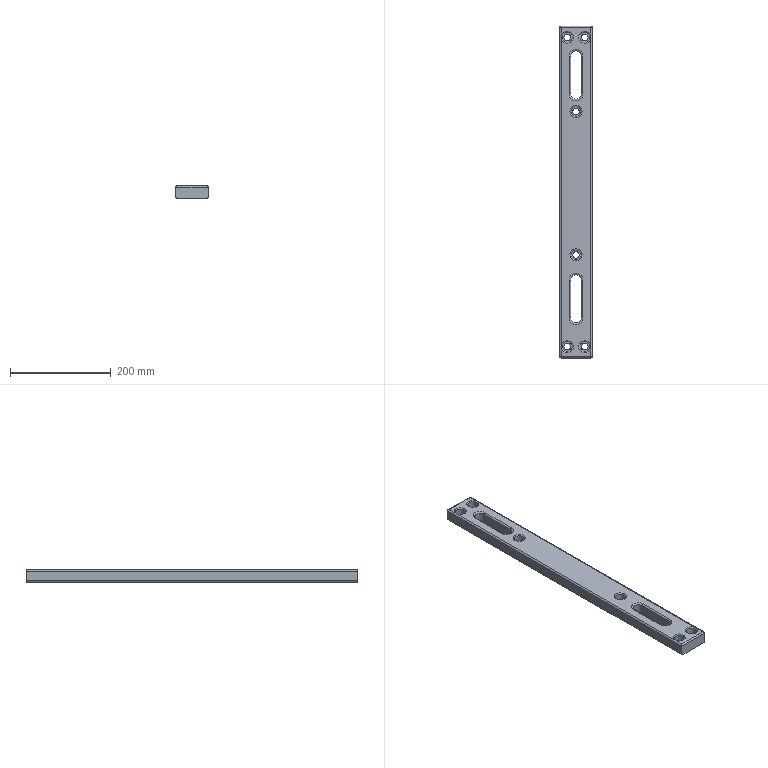Part | NX | features solid 2 | 1 solid | 53 faces | box 65 x 660 x 25 mm | volume 933665 mm3 | cylinder 26 | plane 17 | torus 10 | commonest cylinder face diameters 6 x10 13 x6 20 x6 21 x4
STEP:
#1=CARTESIAN_POINT('',(-465.,-309.,403.));
#2=VERTEX_POINT('',#1);
#3=CARTESIAN_POINT('',(-455.,-309.,403.));
#4=DIRECTION('',(0.,0.,-1.));
#5=DIRECTION('',(-1.,0.,0.));
#6=AXIS2_PLACEMENT_3D('',#3,#4,#5);
#7=CIRCLE('',#6,10.);
#8=EDGE_CURVE('',#2,#2,#7,.T.);
#9=ORIENTED_EDGE('',*,*,#8,.F.);
#10=EDGE_LOOP('',(#9));
#11=FACE_BOUND('',#10,.T.);
#12=CARTESIAN_POINT('',(-445.,-309.,390.));
#13=VERTEX_POINT('',#12);
#14=CARTESIAN_POINT('',(-455.,-309.,390.));
#15=DIRECTION('',(0.,0.,-1.));
#16=DIRECTION('',(1.,0.,0.));
#17=AXIS2_PLACEMENT_3D('',#14,#15,#16);
#18=CIRCLE('',#17,10.);
#19=EDGE_CURVE('',#13,#13,#18,.T.);
#20=ORIENTED_EDGE('',*,*,#19,.T.);
#21=EDGE_LOOP('',(#20));
#22=FACE_BOUND('',#21,.T.);
#23=CARTESIAN_POINT('',(-455.,-309.,390.));
#24=DIRECTION('',(0.,0.,1.));
#25=DIRECTION('',(1.,0.,0.));
#26=AXIS2_PLACEMENT_3D('',#23,#24,#25);
#27=CYLINDRICAL_SURFACE('',#26,10.);
#28=ADVANCED_FACE('',(#11,#22),#27,.F.);
#29=CARTESIAN_POINT('',(-500.,-309.,403.));
#30=VERTEX_POINT('',#29);
#31=CARTESIAN_POINT('',(-490.,-309.,403.));
#32=DIRECTION('',(0.,0.,-1.));
#33=DIRECTION('',(-1.,0.,0.));
#34=AXIS2_PLACEMENT_3D('',#31,#32,#33);
#35=CIRCLE('',#34,10.);
#36=EDGE_CURVE('',#30,#30,#35,.T.);
#37=ORIENTED_EDGE('',*,*,#36,.F.);
#38=EDGE_LOOP('',(#37));
#39=FACE_BOUND('',#38,.T.);
#40=CARTESIAN_POINT('',(-480.,-309.,390.));
#41=VERTEX_POINT('',#40);
#42=CARTESIAN_POINT('',(-490.,-309.,390.));
#43=DIRECTION('',(0.,0.,-1.));
#44=DIRECTION('',(1.,0.,0.));
#45=AXIS2_PLACEMENT_3D('',#42,#43,#44);
#46=CIRCLE('',#45,10.);
#47=EDGE_CURVE('',#41,#41,#46,.T.);
#48=ORIENTED_EDGE('',*,*,#47,.T.);
#49=EDGE_LOOP('',(#48));
#50=FACE_BOUND('',#49,.T.);
#51=CARTESIAN_POINT('',(-490.,-309.,390.));
#52=DIRECTION('',(0.,0.,1.));
#53=DIRECTION('',(1.,0.,0.));
#54=AXIS2_PLACEMENT_3D('',#51,#52,#53);
#55=CYLINDRICAL_SURFACE('',#54,10.);
#56=ADVANCED_FACE('',(#39,#50),#55,.F.);
#57=CARTESIAN_POINT('',(-482.5,-126.5,403.));
#58=VERTEX_POINT('',#57);
#59=CARTESIAN_POINT('',(-472.5,-126.5,403.));
#60=DIRECTION('',(0.,0.,-1.));
#61=DIRECTION('',(-1.,0.,0.));
#62=AXIS2_PLACEMENT_3D('',#59,#60,#61);
#63=CIRCLE('',#62,10.);
#64=EDGE_CURVE('',#58,#58,#63,.T.);
#65=ORIENTED_EDGE('',*,*,#64,.F.);
#66=EDGE_LOOP('',(#65));
#67=FACE_BOUND('',#66,.T.);
#68=CARTESIAN_POINT('',(-462.5,-126.5,390.));
#69=VERTEX_POINT('',#68);
#70=CARTESIAN_POINT('',(-472.5,-126.5,390.));
#71=DIRECTION('',(0.,0.,-1.));
#72=DIRECTION('',(1.,0.,0.));
#73=AXIS2_PLACEMENT_3D('',#70,#71,#72);
#74=CIRCLE('',#73,10.);
#75=EDGE_CURVE('',#69,#69,#74,.T.);
#76=ORIENTED_EDGE('',*,*,#75,.T.);
#77=EDGE_LOOP('',(#76));
#78=FACE_BOUND('',#77,.T.);
#79=CARTESIAN_POINT('',(-472.5,-126.5,390.));
#80=DIRECTION('',(0.,0.,1.));
#81=DIRECTION('',(1.,0.,0.));
#82=AXIS2_PLACEMENT_3D('',#79,#80,#81);
#83=CYLINDRICAL_SURFACE('',#82,10.);
#84=ADVANCED_FACE('',(#67,#78),#83,.F.);
#85=ORIENTED_EDGE('',*,*,#47,.F.);
#86=EDGE_LOOP('',(#85));
#87=FACE_BOUND('',#86,.T.);
#88=CARTESIAN_POINT('',(-483.5,-309.,390.));
#89=VERTEX_POINT('',#88);
#90=CARTESIAN_POINT('',(-490.,-309.,390.));
#91=DIRECTION('',(0.,0.,-1.));
#92=DIRECTION('',(1.,0.,0.));
#93=AXIS2_PLACEMENT_3D('',#90,#91,#92);
#94=CIRCLE('',#93,6.5);
#95=EDGE_CURVE('',#89,#89,#94,.F.);
#96=ORIENTED_EDGE('',*,*,#95,.F.);
#97=EDGE_LOOP('',(#96));
#98=FACE_BOUND('',#97,.T.);
#99=CARTESIAN_POINT('',(-490.,-331.5,390.));
#100=DIRECTION('',(0.,0.,1.));
#101=DIRECTION('',(1.,0.,0.));
#102=AXIS2_PLACEMENT_3D('',#99,#100,#101);
#103=PLANE('',#102);
#104=ADVANCED_FACE('',(#87,#98),#103,.T.);
#105=ORIENTED_EDGE('',*,*,#19,.F.);
#106=EDGE_LOOP('',(#105));
#107=FACE_BOUND('',#106,.T.);
#108=CARTESIAN_POINT('',(-448.5,-309.,390.));
#109=VERTEX_POINT('',#108);
#110=CARTESIAN_POINT('',(-455.,-309.,390.));
#111=DIRECTION('',(0.,0.,-1.));
#112=DIRECTION('',(1.,0.,0.));
#113=AXIS2_PLACEMENT_3D('',#110,#111,#112);
#114=CIRCLE('',#113,6.5);
#115=EDGE_CURVE('',#109,#109,#114,.F.);
#116=ORIENTED_EDGE('',*,*,#115,.F.);
#117=EDGE_LOOP('',(#116));
#118=FACE_BOUND('',#117,.T.);
#119=CARTESIAN_POINT('',(-455.,-331.5,390.));
#120=DIRECTION('',(0.,0.,1.));
#121=DIRECTION('',(1.,0.,0.));
#122=AXIS2_PLACEMENT_3D('',#119,#120,#121);
#123=PLANE('',#122);
#124=ADVANCED_FACE('',(#107,#118),#123,.T.);
#125=ORIENTED_EDGE('',*,*,#75,.F.);
#126=EDGE_LOOP('',(#125));
#127=FACE_BOUND('',#126,.T.);
#128=CARTESIAN_POINT('',(-466.,-126.5,390.));
#129=VERTEX_POINT('',#128);
#130=CARTESIAN_POINT('',(-472.5,-126.5,390.));
#131=DIRECTION('',(0.,0.,-1.));
#132=DIRECTION('',(1.,0.,0.));
#133=AXIS2_PLACEMENT_3D('',#130,#131,#132);
#134=CIRCLE('',#133,6.5);
#135=EDGE_CURVE('',#129,#129,#134,.F.);
#136=ORIENTED_EDGE('',*,*,#135,.F.);
#137=EDGE_LOOP('',(#136));
#138=FACE_BOUND('',#137,.T.);
#139=CARTESIAN_POINT('',(-472.5,-128.,390.));
#140=DIRECTION('',(0.,0.,1.));
#141=DIRECTION('',(1.,0.,0.));
#142=AXIS2_PLACEMENT_3D('',#139,#140,#141);
#143=PLANE('',#142);
#144=ADVANCED_FACE('',(#127,#138),#143,.T.);
#145=CARTESIAN_POINT('',(-443.,-309.007,405.));
#146=VERTEX_POINT('',#145);
#147=CARTESIAN_POINT('',(-455.,-309.,405.));
#148=DIRECTION('',(0.,0.,-1.));
#149=DIRECTION('',(-1.,0.,0.));
#150=AXIS2_PLACEMENT_3D('',#147,#148,#149);
#151=CIRCLE('',#150,12.);
#152=EDGE_CURVE('',#146,#146,#151,.F.);
#153=ORIENTED_EDGE('',*,*,#152,.T.);
#154=EDGE_LOOP('',(#153));
#155=FACE_BOUND('',#154,.T.);
#156=ORIENTED_EDGE('',*,*,#8,.T.);
#157=EDGE_LOOP('',(#156));
#158=FACE_BOUND('',#157,.T.);
#159=CARTESIAN_POINT('',(-455.,-309.,403.));
#160=DIRECTION('',(0.,0.,1.));
#161=DIRECTION('',(-1.,0.,0.));
#162=AXIS2_PLACEMENT_3D('',#159,#160,#161);
#163=TOROIDAL_SURFACE('',#162,12.,2.);
#164=ADVANCED_FACE('',(#155,#158),#163,.T.);
#165=CARTESIAN_POINT('',(-502.,-309.007,405.));
#166=VERTEX_POINT('',#165);
#167=CARTESIAN_POINT('',(-490.,-309.,405.));
#168=DIRECTION('',(0.,0.,-1.));
#169=DIRECTION('',(-1.,0.,0.));
#170=AXIS2_PLACEMENT_3D('',#167,#168,#169);
#171=CIRCLE('',#170,12.);
#172=EDGE_CURVE('',#166,#166,#171,.F.);
#173=ORIENTED_EDGE('',*,*,#172,.T.);
#174=EDGE_LOOP('',(#173));
#175=FACE_BOUND('',#174,.T.);
#176=ORIENTED_EDGE('',*,*,#36,.T.);
#177=EDGE_LOOP('',(#176));
#178=FACE_BOUND('',#177,.T.);
#179=CARTESIAN_POINT('',(-490.,-309.,403.));
#180=DIRECTION('',(0.,0.,1.));
#181=DIRECTION('',(-1.,0.,0.));
#182=AXIS2_PLACEMENT_3D('',#179,#180,#181);
#183=TOROIDAL_SURFACE('',#182,12.,2.);
#184=ADVANCED_FACE('',(#175,#178),#183,.T.);
#185=CARTESIAN_POINT('',(-484.5,-126.5,405.));
#186=VERTEX_POINT('',#185);
#187=CARTESIAN_POINT('',(-472.5,-126.5,405.));
#188=DIRECTION('',(0.,0.,-1.));
#189=DIRECTION('',(-1.,0.,0.));
#190=AXIS2_PLACEMENT_3D('',#187,#188,#189);
#191=CIRCLE('',#190,12.);
#192=EDGE_CURVE('',#186,#186,#191,.F.);
#193=ORIENTED_EDGE('',*,*,#192,.T.);
#194=EDGE_LOOP('',(#193));
#195=FACE_BOUND('',#194,.T.);
#196=ORIENTED_EDGE('',*,*,#64,.T.);
#197=EDGE_LOOP('',(#196));
#198=FACE_BOUND('',#197,.T.);
#199=CARTESIAN_POINT('',(-472.5,-126.5,403.));
#200=DIRECTION('',(0.,0.,1.));
#201=DIRECTION('',(-1.,0.,0.));
#202=AXIS2_PLACEMENT_3D('',#199,#200,#201);
#203=TOROIDAL_SURFACE('',#202,12.,2.);
#204=ADVANCED_FACE('',(#195,#198),#203,.T.);
#205=CARTESIAN_POINT('',(-483.,-251.5,402.));
#206=VERTEX_POINT('',#205);
#207=CARTESIAN_POINT('',(-486.,-251.5,405.));
#208=VERTEX_POINT('',#207);
#209=CARTESIAN_POINT('',(-486.,-251.5,402.));
#210=DIRECTION('',(0.,-1.,0.));
#211=DIRECTION('',(0.,0.,1.));
#212=AXIS2_PLACEMENT_3D('',#209,#210,#211);
#213=CIRCLE('',#212,3.);
#214=EDGE_CURVE('',#206,#208,#213,.T.);
#215=ORIENTED_EDGE('',*,*,#214,.F.);
#216=CARTESIAN_POINT('',(-483.,-176.5,402.));
#217=VERTEX_POINT('',#216);
#218=CARTESIAN_POINT('',(-483.,-249.,402.));
#219=DIRECTION('',(0.,1.,0.));
#220=VECTOR('',#219,1000.);
#221=LINE('',#218,#220);
#222=EDGE_CURVE('',#206,#217,#221,.T.);
#223=ORIENTED_EDGE('',*,*,#222,.T.);
#224=CARTESIAN_POINT('',(-486.,-176.5,405.));
#225=VERTEX_POINT('',#224);
#226=CARTESIAN_POINT('',(-486.,-176.5,402.));
#227=DIRECTION('',(0.,1.,0.));
#228=DIRECTION('',(0.,0.,-1.));
#229=AXIS2_PLACEMENT_3D('',#226,#227,#228);
#230=CIRCLE('',#229,3.);
#231=EDGE_CURVE('',#225,#217,#230,.T.);
#232=ORIENTED_EDGE('',*,*,#231,.F.);
#233=CARTESIAN_POINT('',(-486.,353.5,405.));
#234=DIRECTION('',(0.,1.,0.));
#235=VECTOR('',#234,1000.);
#236=LINE('',#233,#235);
#237=EDGE_CURVE('',#225,#208,#236,.F.);
#238=ORIENTED_EDGE('',*,*,#237,.T.);
#239=EDGE_LOOP('',(#215,#223,#232,#238));
#240=FACE_BOUND('',#239,.T.);
#241=CARTESIAN_POINT('',(-486.,-249.,402.));
#242=DIRECTION('',(0.,1.,0.));
#243=DIRECTION('',(0.,0.,1.));
#244=AXIS2_PLACEMENT_3D('',#241,#242,#243);
#245=CYLINDRICAL_SURFACE('',#244,3.);
#246=ADVANCED_FACE('',(#240),#245,.T.);
#247=CARTESIAN_POINT('',(-462.,-251.5,402.));
#248=VERTEX_POINT('',#247);
#249=CARTESIAN_POINT('',(-459.,-251.5,405.));
#250=VERTEX_POINT('',#249);
#251=CARTESIAN_POINT('',(-459.,-251.5,402.));
#252=DIRECTION('',(0.,1.,0.));
#253=DIRECTION('',(0.,0.,-1.));
#254=AXIS2_PLACEMENT_3D('',#251,#252,#253);
#255=CIRCLE('',#254,3.);
#256=EDGE_CURVE('',#248,#250,#255,.T.);
#257=ORIENTED_EDGE('',*,*,#256,.F.);
#258=CARTESIAN_POINT('',(-472.5,-251.5,402.));
#259=DIRECTION('',(0.,0.,-1.));
#260=DIRECTION('',(-1.,0.,0.));
#261=AXIS2_PLACEMENT_3D('',#258,#259,#260);
#262=CIRCLE('',#261,10.5);
#263=EDGE_CURVE('',#248,#206,#262,.T.);
#264=ORIENTED_EDGE('',*,*,#263,.T.);
#265=ORIENTED_EDGE('',*,*,#214,.T.);
#266=CARTESIAN_POINT('',(-472.5,-251.5,405.));
#267=DIRECTION('',(0.,0.,-1.));
#268=DIRECTION('',(-1.,0.,0.));
#269=AXIS2_PLACEMENT_3D('',#266,#267,#268);
#270=CIRCLE('',#269,13.5);
#271=EDGE_CURVE('',#208,#250,#270,.F.);
#272=ORIENTED_EDGE('',*,*,#271,.T.);
#273=EDGE_LOOP('',(#257,#264,#265,#272));
#274=FACE_BOUND('',#273,.T.);
#275=CARTESIAN_POINT('',(-472.5,-251.5,402.));
#276=DIRECTION('',(0.,0.,1.));
#277=DIRECTION('',(-1.,0.,0.));
#278=AXIS2_PLACEMENT_3D('',#275,#276,#277);
#279=TOROIDAL_SURFACE('',#278,13.5,3.);
#280=ADVANCED_FACE('',(#274),#279,.T.);
#281=CARTESIAN_POINT('',(-459.,-176.5,405.));
#282=VERTEX_POINT('',#281);
#283=CARTESIAN_POINT('',(-462.,-176.5,402.));
#284=VERTEX_POINT('',#283);
#285=CARTESIAN_POINT('',(-459.,-176.5,402.));
#286=DIRECTION('',(0.,-1.,0.));
#287=DIRECTION('',(0.,0.,1.));
#288=AXIS2_PLACEMENT_3D('',#285,#286,#287);
#289=CIRCLE('',#288,3.);
#290=EDGE_CURVE('',#282,#284,#289,.T.);
#291=ORIENTED_EDGE('',*,*,#290,.T.);
#292=CARTESIAN_POINT('',(-462.,-178.,402.));
#293=DIRECTION('',(0.,-1.,0.));
#294=VECTOR('',#293,1000.);
#295=LINE('',#292,#294);
#296=EDGE_CURVE('',#284,#248,#295,.T.);
#297=ORIENTED_EDGE('',*,*,#296,.T.);
#298=ORIENTED_EDGE('',*,*,#256,.T.);
#299=CARTESIAN_POINT('',(-459.,353.5,405.));
#300=DIRECTION('',(0.,-1.,0.));
#301=VECTOR('',#300,1000.);
#302=LINE('',#299,#301);
#303=EDGE_CURVE('',#250,#282,#302,.F.);
#304=ORIENTED_EDGE('',*,*,#303,.T.);
#305=EDGE_LOOP('',(#291,#297,#298,#304));
#306=FACE_BOUND('',#305,.T.);
#307=CARTESIAN_POINT('',(-459.,-178.,402.));
#308=DIRECTION('',(0.,-1.,0.));
#309=DIRECTION('',(0.,0.,-1.));
#310=AXIS2_PLACEMENT_3D('',#307,#308,#309);
#311=CYLINDRICAL_SURFACE('',#310,3.);
#312=ADVANCED_FACE('',(#306),#311,.T.);
#313=ORIENTED_EDGE('',*,*,#290,.F.);
#314=CARTESIAN_POINT('',(-472.5,-176.5,405.));
#315=DIRECTION('',(0.,0.,-1.));
#316=DIRECTION('',(-1.,0.,0.));
#317=AXIS2_PLACEMENT_3D('',#314,#315,#316);
#318=CIRCLE('',#317,13.5);
#319=EDGE_CURVE('',#282,#225,#318,.F.);
#320=ORIENTED_EDGE('',*,*,#319,.T.);
#321=ORIENTED_EDGE('',*,*,#231,.T.);
#322=CARTESIAN_POINT('',(-472.5,-176.5,402.));
#323=DIRECTION('',(0.,0.,-1.));
#324=DIRECTION('',(-1.,0.,0.));
#325=AXIS2_PLACEMENT_3D('',#322,#323,#324);
#326=CIRCLE('',#325,10.5);
#327=EDGE_CURVE('',#217,#284,#326,.T.);
#328=ORIENTED_EDGE('',*,*,#327,.T.);
#329=EDGE_LOOP('',(#313,#320,#321,#328));
#330=FACE_BOUND('',#329,.T.);
#331=CARTESIAN_POINT('',(-472.5,-176.5,402.));
#332=DIRECTION('',(0.,0.,1.));
#333=DIRECTION('',(-1.,0.,0.));
#334=AXIS2_PLACEMENT_3D('',#331,#332,#333);
#335=TOROIDAL_SURFACE('',#334,13.5,3.);
#336=ADVANCED_FACE('',(#330),#335,.T.);
#337=CARTESIAN_POINT('',(-462.,-251.5,380.));
#338=VERTEX_POINT('',#337);
#339=CARTESIAN_POINT('',(-462.,-251.5,405.));
#340=DIRECTION('',(0.,0.,-1.));
#341=VECTOR('',#340,1000.);
#342=LINE('',#339,#341);
#343=EDGE_CURVE('',#248,#338,#342,.T.);
#344=ORIENTED_EDGE('',*,*,#343,.T.);
#345=CARTESIAN_POINT('',(-483.,-251.5,380.));
#346=VERTEX_POINT('',#345);
#347=CARTESIAN_POINT('',(-472.5,-251.5,380.));
#348=DIRECTION('',(0.,0.,-1.));
#349=DIRECTION('',(1.,0.,0.));
#350=AXIS2_PLACEMENT_3D('',#347,#348,#349);
#351=CIRCLE('',#350,10.5);
#352=EDGE_CURVE('',#338,#346,#351,.T.);
#353=ORIENTED_EDGE('',*,*,#352,.T.);
#354=CARTESIAN_POINT('',(-483.,-251.5,405.));
#355=DIRECTION('',(0.,0.,-1.));
#356=VECTOR('',#355,1000.);
#357=LINE('',#354,#356);
#358=EDGE_CURVE('',#206,#346,#357,.T.);
#359=ORIENTED_EDGE('',*,*,#358,.F.);
#360=ORIENTED_EDGE('',*,*,#263,.F.);
#361=EDGE_LOOP('',(#344,#353,#359,#360));
#362=FACE_BOUND('',#361,.T.);
#363=CARTESIAN_POINT('',(-472.5,-251.5,405.));
#364=DIRECTION('',(0.,0.,-1.));
#365=DIRECTION('',(-1.,0.,0.));
#366=AXIS2_PLACEMENT_3D('',#363,#364,#365);
#367=CYLINDRICAL_SURFACE('',#366,10.5);
#368=ADVANCED_FACE('',(#362),#367,.F.);
#369=ORIENTED_EDGE('',*,*,#358,.T.);
#370=CARTESIAN_POINT('',(-483.,-176.5,380.));
#371=VERTEX_POINT('',#370);
#372=CARTESIAN_POINT('',(-483.,-249.,380.));
#373=DIRECTION('',(0.,1.,0.));
#374=VECTOR('',#373,1000.);
#375=LINE('',#372,#374);
#376=EDGE_CURVE('',#346,#371,#375,.T.);
#377=ORIENTED_EDGE('',*,*,#376,.T.);
#378=CARTESIAN_POINT('',(-483.,-176.5,405.));
#379=DIRECTION('',(0.,0.,-1.));
#380=VECTOR('',#379,1000.);
#381=LINE('',#378,#380);
#382=EDGE_CURVE('',#217,#371,#381,.T.);
#383=ORIENTED_EDGE('',*,*,#382,.F.);
#384=ORIENTED_EDGE('',*,*,#222,.F.);
#385=EDGE_LOOP('',(#369,#377,#383,#384));
#386=FACE_BOUND('',#385,.T.);
#387=CARTESIAN_POINT('',(-483.,-249.,405.));
#388=DIRECTION('',(1.,0.,0.));
#389=DIRECTION('',(0.,0.,-1.));
#390=AXIS2_PLACEMENT_3D('',#387,#388,#389);
#391=PLANE('',#390);
#392=ADVANCED_FACE('',(#386),#391,.T.);
#393=ORIENTED_EDGE('',*,*,#382,.T.);
#394=CARTESIAN_POINT('',(-462.,-176.5,380.));
#395=VERTEX_POINT('',#394);
#396=CARTESIAN_POINT('',(-472.5,-176.5,380.));
#397=DIRECTION('',(0.,0.,-1.));
#398=DIRECTION('',(1.,0.,0.));
#399=AXIS2_PLACEMENT_3D('',#396,#397,#398);
#400=CIRCLE('',#399,10.5);
#401=EDGE_CURVE('',#371,#395,#400,.T.);
#402=ORIENTED_EDGE('',*,*,#401,.T.);
#403=CARTESIAN_POINT('',(-462.,-176.5,405.));
#404=DIRECTION('',(0.,0.,-1.));
#405=VECTOR('',#404,1000.);
#406=LINE('',#403,#405);
#407=EDGE_CURVE('',#284,#395,#406,.T.);
#408=ORIENTED_EDGE('',*,*,#407,.F.);
#409=ORIENTED_EDGE('',*,*,#327,.F.);
#410=EDGE_LOOP('',(#393,#402,#408,#409));
#411=FACE_BOUND('',#410,.T.);
#412=CARTESIAN_POINT('',(-472.5,-176.5,405.));
#413=DIRECTION('',(0.,0.,-1.));
#414=DIRECTION('',(-1.,0.,0.));
#415=AXIS2_PLACEMENT_3D('',#412,#413,#414);
#416=CYLINDRICAL_SURFACE('',#415,10.5);
#417=ADVANCED_FACE('',(#411),#416,.F.);
#418=ORIENTED_EDGE('',*,*,#407,.T.);
#419=CARTESIAN_POINT('',(-462.,-178.,380.));
#420=DIRECTION('',(0.,-1.,0.));
#421=VECTOR('',#420,1000.);
#422=LINE('',#419,#421);
#423=EDGE_CURVE('',#395,#338,#422,.T.);
#424=ORIENTED_EDGE('',*,*,#423,.T.);
#425=ORIENTED_EDGE('',*,*,#343,.F.);
#426=ORIENTED_EDGE('',*,*,#296,.F.);
#427=EDGE_LOOP('',(#418,#424,#425,#426));
#428=FACE_BOUND('',#427,.T.);
#429=CARTESIAN_POINT('',(-462.,-178.,405.));
#430=DIRECTION('',(-1.,0.,0.));
#431=DIRECTION('',(0.,0.,1.));
#432=AXIS2_PLACEMENT_3D('',#429,#430,#431);
#433=PLANE('',#432);
#434=ADVANCED_FACE('',(#428),#433,.T.);
#435=CARTESIAN_POINT('',(-483.5,-309.,380.));
#436=VERTEX_POINT('',#435);
#437=CARTESIAN_POINT('',(-490.,-309.,380.));
#438=DIRECTION('',(0.,0.,-1.));
#439=DIRECTION('',(1.,0.,0.));
#440=AXIS2_PLACEMENT_3D('',#437,#438,#439);
#441=CIRCLE('',#440,6.5);
#442=EDGE_CURVE('',#436,#436,#441,.T.);
#443=ORIENTED_EDGE('',*,*,#442,.T.);
#444=EDGE_LOOP('',(#443));
#445=FACE_BOUND('',#444,.T.);
#446=ORIENTED_EDGE('',*,*,#95,.T.);
#447=EDGE_LOOP('',(#446));
#448=FACE_BOUND('',#447,.T.);
#449=CARTESIAN_POINT('',(-490.,-309.,380.));
#450=DIRECTION('',(0.,0.,1.));
#451=DIRECTION('',(1.,0.,0.));
#452=AXIS2_PLACEMENT_3D('',#449,#450,#451);
#453=CYLINDRICAL_SURFACE('',#452,6.5);
#454=ADVANCED_FACE('',(#445,#448),#453,.F.);
#455=CARTESIAN_POINT('',(-448.5,-309.,380.));
#456=VERTEX_POINT('',#455);
#457=CARTESIAN_POINT('',(-455.,-309.,380.));
#458=DIRECTION('',(0.,0.,-1.));
#459=DIRECTION('',(1.,0.,0.));
#460=AXIS2_PLACEMENT_3D('',#457,#458,#459);
#461=CIRCLE('',#460,6.5);
#462=EDGE_CURVE('',#456,#456,#461,.T.);
#463=ORIENTED_EDGE('',*,*,#462,.T.);
#464=EDGE_LOOP('',(#463));
#465=FACE_BOUND('',#464,.T.);
#466=ORIENTED_EDGE('',*,*,#115,.T.);
#467=EDGE_LOOP('',(#466));
#468=FACE_BOUND('',#467,.T.);
#469=CARTESIAN_POINT('',(-455.,-309.,380.));
#470=DIRECTION('',(0.,0.,1.));
#471=DIRECTION('',(1.,0.,0.));
#472=AXIS2_PLACEMENT_3D('',#469,#470,#471);
#473=CYLINDRICAL_SURFACE('',#472,6.5);
#474=ADVANCED_FACE('',(#465,#468),#473,.F.);
#475=CARTESIAN_POINT('',(-466.,-126.5,380.));
#476=VERTEX_POINT('',#475);
#477=CARTESIAN_POINT('',(-472.5,-126.5,380.));
#478=DIRECTION('',(0.,0.,-1.));
#479=DIRECTION('',(1.,0.,0.));
#480=AXIS2_PLACEMENT_3D('',#477,#478,#479);
#481=CIRCLE('',#480,6.5);
#482=EDGE_CURVE('',#476,#476,#481,.T.);
#483=ORIENTED_EDGE('',*,*,#482,.T.);
#484=EDGE_LOOP('',(#483));
#485=FACE_BOUND('',#484,.T.);
#486=ORIENTED_EDGE('',*,*,#135,.T.);
#487=EDGE_LOOP('',(#486));
#488=FACE_BOUND('',#487,.T.);
#489=CARTESIAN_POINT('',(-472.5,-126.5,380.));
#490=DIRECTION('',(0.,0.,1.));
#491=DIRECTION('',(1.,0.,0.));
#492=AXIS2_PLACEMENT_3D('',#489,#490,#491);
#493=CYLINDRICAL_SURFACE('',#492,6.5);
#494=ADVANCED_FACE('',(#485,#488),#493,.F.);
#495=CARTESIAN_POINT('',(-505.,-331.5,402.));
#496=VERTEX_POINT('',#495);
#497=CARTESIAN_POINT('',(-502.,-328.5,405.));
#498=VERTEX_POINT('',#497);
#499=CARTESIAN_POINT('',(-502.,-328.5,402.));
#500=DIRECTION('',(-0.7071,0.7071,0.));
#501=DIRECTION('',(0.7071,0.7071,0.));
#502=AXIS2_PLACEMENT_3D('',#499,#500,#501);
#503=ELLIPSE('',#502,4.243,3.);
#504=EDGE_CURVE('',#496,#498,#503,.T.);
#505=ORIENTED_EDGE('',*,*,#504,.F.);
#506=CARTESIAN_POINT('',(-440.,-331.5,402.));
#507=VERTEX_POINT('',#506);
#508=CARTESIAN_POINT('',(-605.,-331.5,402.));
#509=DIRECTION('',(-1.,0.,0.));
#510=VECTOR('',#509,1000.);
#511=LINE('',#508,#510);
#512=EDGE_CURVE('',#496,#507,#511,.F.);
#513=ORIENTED_EDGE('',*,*,#512,.T.);
#514=CARTESIAN_POINT('',(-443.,-328.5,405.));
#515=VERTEX_POINT('',#514);
#516=CARTESIAN_POINT('',(-443.,-328.5,402.));
#517=DIRECTION('',(-0.7071,-0.7071,0.));
#518=DIRECTION('',(0.7071,-0.7071,0.));
#519=AXIS2_PLACEMENT_3D('',#516,#517,#518);
#520=ELLIPSE('',#519,4.243,3.);
#521=EDGE_CURVE('',#507,#515,#520,.T.);
#522=ORIENTED_EDGE('',*,*,#521,.T.);
#523=CARTESIAN_POINT('',(-505.,-328.5,405.));
#524=DIRECTION('',(1.,0.,0.));
#525=VECTOR('',#524,1000.);
#526=LINE('',#523,#525);
#527=EDGE_CURVE('',#515,#498,#526,.F.);
#528=ORIENTED_EDGE('',*,*,#527,.T.);
#529=EDGE_LOOP('',(#505,#513,#522,#528));
#530=FACE_BOUND('',#529,.T.);
#531=CARTESIAN_POINT('',(-505.,-328.5,402.));
#532=DIRECTION('',(1.,0.,0.));
#533=DIRECTION('',(0.,0.,1.));
#534=AXIS2_PLACEMENT_3D('',#531,#532,#533);
#535=CYLINDRICAL_SURFACE('',#534,3.);
#536=ADVANCED_FACE('',(#530),#535,.T.);
#537=CARTESIAN_POINT('',(-440.,-331.5,383.));
#538=VERTEX_POINT('',#537);
#539=CARTESIAN_POINT('',(-440.,-331.5,405.));
#540=DIRECTION('',(0.,0.,1.));
#541=VECTOR('',#540,1000.);
#542=LINE('',#539,#541);
#543=EDGE_CURVE('',#507,#538,#542,.F.);
#544=ORIENTED_EDGE('',*,*,#543,.F.);
#545=ORIENTED_EDGE('',*,*,#512,.F.);
#546=CARTESIAN_POINT('',(-505.,-331.5,383.));
#547=VERTEX_POINT('',#546);
#548=CARTESIAN_POINT('',(-505.,-331.5,320.));
#549=DIRECTION('',(0.,0.,1.));
#550=VECTOR('',#549,1000.);
#551=LINE('',#548,#550);
#552=EDGE_CURVE('',#496,#547,#551,.F.);
#553=ORIENTED_EDGE('',*,*,#552,.T.);
#554=CARTESIAN_POINT('',(-502.,-331.5,380.));
#555=VERTEX_POINT('',#554);
#556=CARTESIAN_POINT('',(-502.,-331.5,383.));
#557=DIRECTION('',(0.,-1.,0.));
#558=DIRECTION('',(0.,0.,1.));
#559=AXIS2_PLACEMENT_3D('',#556,#557,#558);
#560=CIRCLE('',#559,3.);
#561=EDGE_CURVE('',#555,#547,#560,.F.);
#562=ORIENTED_EDGE('',*,*,#561,.F.);
#563=CARTESIAN_POINT('',(-443.,-331.5,380.));
#564=VERTEX_POINT('',#563);
#565=CARTESIAN_POINT('',(-505.,-331.5,380.));
#566=DIRECTION('',(1.,0.,0.));
#567=VECTOR('',#566,1000.);
#568=LINE('',#565,#567);
#569=EDGE_CURVE('',#564,#555,#568,.F.);
#570=ORIENTED_EDGE('',*,*,#569,.F.);
#571=CARTESIAN_POINT('',(-443.,-331.5,383.));
#572=DIRECTION('',(0.,-1.,0.));
#573=DIRECTION('',(0.,0.,1.));
#574=AXIS2_PLACEMENT_3D('',#571,#572,#573);
#575=CIRCLE('',#574,3.);
#576=EDGE_CURVE('',#538,#564,#575,.F.);
#577=ORIENTED_EDGE('',*,*,#576,.F.);
#578=EDGE_LOOP('',(#544,#545,#553,#562,#570,#577));
#579=FACE_BOUND('',#578,.T.);
#580=CARTESIAN_POINT('',(-605.,-331.5,320.));
#581=DIRECTION('',(0.,1.,0.));
#582=DIRECTION('',(0.,0.,-1.));
#583=AXIS2_PLACEMENT_3D('',#580,#581,#582);
#584=PLANE('',#583);
#585=ADVANCED_FACE('',(#579),#584,.F.);
#586=CARTESIAN_POINT('',(-505.,328.5,383.));
#587=VERTEX_POINT('',#586);
#588=CARTESIAN_POINT('',(-505.,-371.5,383.));
#589=DIRECTION('',(0.,1.,0.));
#590=VECTOR('',#589,1000.);
#591=LINE('',#588,#590);
#592=EDGE_CURVE('',#547,#587,#591,.T.);
#593=ORIENTED_EDGE('',*,*,#592,.T.);
#594=CARTESIAN_POINT('',(-502.,328.5,380.));
#595=VERTEX_POINT('',#594);
#596=CARTESIAN_POINT('',(-502.,328.5,383.));
#597=DIRECTION('',(0.,1.,0.));
#598=DIRECTION('',(0.,0.,-1.));
#599=AXIS2_PLACEMENT_3D('',#596,#597,#598);
#600=CIRCLE('',#599,3.);
#601=EDGE_CURVE('',#587,#595,#600,.F.);
#602=ORIENTED_EDGE('',*,*,#601,.T.);
#603=CARTESIAN_POINT('',(-502.,353.5,380.));
#604=DIRECTION('',(0.,1.,0.));
#605=VECTOR('',#604,1000.);
#606=LINE('',#603,#605);
#607=EDGE_CURVE('',#595,#555,#606,.F.);
#608=ORIENTED_EDGE('',*,*,#607,.T.);
#609=ORIENTED_EDGE('',*,*,#561,.T.);
#610=EDGE_LOOP('',(#593,#602,#608,#609));
#611=FACE_BOUND('',#610,.T.);
#612=CARTESIAN_POINT('',(-502.,-371.5,383.));
#613=DIRECTION('',(0.,1.,0.));
#614=DIRECTION('',(0.,0.,1.));
#615=AXIS2_PLACEMENT_3D('',#612,#613,#614);
#616=CYLINDRICAL_SURFACE('',#615,3.);
#617=ADVANCED_FACE('',(#611),#616,.T.);
#618=CARTESIAN_POINT('',(-443.,328.5,380.));
#619=VERTEX_POINT('',#618);
#620=CARTESIAN_POINT('',(-443.,353.5,380.));
#621=DIRECTION('',(0.,-1.,0.));
#622=VECTOR('',#621,1000.);
#623=LINE('',#620,#622);
#624=EDGE_CURVE('',#564,#619,#623,.F.);
#625=ORIENTED_EDGE('',*,*,#624,.T.);
#626=CARTESIAN_POINT('',(-440.,328.5,383.));
#627=VERTEX_POINT('',#626);
#628=CARTESIAN_POINT('',(-443.,328.5,383.));
#629=DIRECTION('',(0.,1.,0.));
#630=DIRECTION('',(0.,0.,-1.));
#631=AXIS2_PLACEMENT_3D('',#628,#629,#630);
#632=CIRCLE('',#631,3.);
#633=EDGE_CURVE('',#619,#627,#632,.F.);
#634=ORIENTED_EDGE('',*,*,#633,.T.);
#635=CARTESIAN_POINT('',(-440.,353.5,383.));
#636=DIRECTION('',(0.,-1.,0.));
#637=VECTOR('',#636,1000.);
#638=LINE('',#635,#637);
#639=EDGE_CURVE('',#627,#538,#638,.T.);
#640=ORIENTED_EDGE('',*,*,#639,.T.);
#641=ORIENTED_EDGE('',*,*,#576,.T.);
#642=EDGE_LOOP('',(#625,#634,#640,#641));
#643=FACE_BOUND('',#642,.T.);
#644=CARTESIAN_POINT('',(-443.,353.5,383.));
#645=DIRECTION('',(0.,-1.,0.));
#646=DIRECTION('',(0.,0.,-1.));
#647=AXIS2_PLACEMENT_3D('',#644,#645,#646);
#648=CYLINDRICAL_SURFACE('',#647,3.);
#649=ADVANCED_FACE('',(#643),#648,.T.);
#650=ORIENTED_EDGE('',*,*,#482,.F.);
#651=EDGE_LOOP('',(#650));
#652=FACE_BOUND('',#651,.T.);
#653=ORIENTED_EDGE('',*,*,#462,.F.);
#654=EDGE_LOOP('',(#653));
#655=FACE_BOUND('',#654,.T.);
#656=ORIENTED_EDGE('',*,*,#442,.F.);
#657=EDGE_LOOP('',(#656));
#658=FACE_BOUND('',#657,.T.);
#659=ORIENTED_EDGE('',*,*,#423,.F.);
#660=ORIENTED_EDGE('',*,*,#401,.F.);
#661=ORIENTED_EDGE('',*,*,#376,.F.);
#662=ORIENTED_EDGE('',*,*,#352,.F.);
#663=EDGE_LOOP('',(#659,#660,#661,#662));
#664=FACE_BOUND('',#663,.T.);
#665=ORIENTED_EDGE('',*,*,#607,.F.);
#666=CARTESIAN_POINT('',(-505.,328.5,380.));
#667=DIRECTION('',(-1.,0.,0.));
#668=VECTOR('',#667,1000.);
#669=LINE('',#666,#668);
#670=EDGE_CURVE('',#595,#619,#669,.F.);
#671=ORIENTED_EDGE('',*,*,#670,.T.);
#672=ORIENTED_EDGE('',*,*,#624,.F.);
#673=ORIENTED_EDGE('',*,*,#569,.T.);
#674=EDGE_LOOP('',(#665,#671,#672,#673));
#675=FACE_BOUND('',#674,.T.);
#676=CARTESIAN_POINT('',(-461.5,306.,380.));
#677=VERTEX_POINT('',#676);
#678=CARTESIAN_POINT('',(-455.,306.,380.));
#679=DIRECTION('',(0.,0.,1.));
#680=DIRECTION('',(-1.,0.,0.));
#681=AXIS2_PLACEMENT_3D('',#678,#679,#680);
#682=CIRCLE('',#681,6.5);
#683=EDGE_CURVE('',#677,#677,#682,.T.);
#684=ORIENTED_EDGE('',*,*,#683,.T.);
#685=EDGE_LOOP('',(#684));
#686=FACE_BOUND('',#685,.T.);
#687=CARTESIAN_POINT('',(-496.5,306.,380.));
#688=VERTEX_POINT('',#687);
#689=CARTESIAN_POINT('',(-490.,306.,380.));
#690=DIRECTION('',(0.,0.,1.));
#691=DIRECTION('',(-1.,0.,0.));
#692=AXIS2_PLACEMENT_3D('',#689,#690,#691);
#693=CIRCLE('',#692,6.5);
#694=EDGE_CURVE('',#688,#688,#693,.T.);
#695=ORIENTED_EDGE('',*,*,#694,.T.);
#696=EDGE_LOOP('',(#695));
#697=FACE_BOUND('',#696,.T.);
#698=CARTESIAN_POINT('',(-466.,158.5,380.));
#699=VERTEX_POINT('',#698);
#700=CARTESIAN_POINT('',(-472.5,158.5,380.));
#701=DIRECTION('',(0.,0.,-1.));
#702=DIRECTION('',(1.,0.,0.));
#703=AXIS2_PLACEMENT_3D('',#700,#701,#702);
#704=CIRCLE('',#703,6.5);
#705=EDGE_CURVE('',#699,#699,#704,.T.);
#706=ORIENTED_EDGE('',*,*,#705,.F.);
#707=EDGE_LOOP('',(#706));
#708=FACE_BOUND('',#707,.T.);
#709=CARTESIAN_POINT('',(-483.,193.5,380.));
#710=VERTEX_POINT('',#709);
#711=CARTESIAN_POINT('',(-483.,268.5,380.));
#712=VERTEX_POINT('',#711);
#713=CARTESIAN_POINT('',(-483.,208.,380.));
#714=DIRECTION('',(0.,1.,0.));
#715=VECTOR('',#714,1000.);
#716=LINE('',#713,#715);
#717=EDGE_CURVE('',#710,#712,#716,.T.);
#718=ORIENTED_EDGE('',*,*,#717,.F.);
#719=CARTESIAN_POINT('',(-462.,193.5,380.));
#720=VERTEX_POINT('',#719);
#721=CARTESIAN_POINT('',(-472.5,193.5,380.));
#722=DIRECTION('',(0.,0.,-1.));
#723=DIRECTION('',(1.,0.,0.));
#724=AXIS2_PLACEMENT_3D('',#721,#722,#723);
#725=CIRCLE('',#724,10.5);
#726=EDGE_CURVE('',#720,#710,#725,.T.);
#727=ORIENTED_EDGE('',*,*,#726,.F.);
#728=CARTESIAN_POINT('',(-462.,268.5,380.));
#729=VERTEX_POINT('',#728);
#730=CARTESIAN_POINT('',(-462.,279.,380.));
#731=DIRECTION('',(0.,-1.,0.));
#732=VECTOR('',#731,1000.);
#733=LINE('',#730,#732);
#734=EDGE_CURVE('',#729,#720,#733,.T.);
#735=ORIENTED_EDGE('',*,*,#734,.F.);
#736=CARTESIAN_POINT('',(-472.5,268.5,380.));
#737=DIRECTION('',(0.,0.,-1.));
#738=DIRECTION('',(1.,0.,0.));
#739=AXIS2_PLACEMENT_3D('',#736,#737,#738);
#740=CIRCLE('',#739,10.5);
#741=EDGE_CURVE('',#712,#729,#740,.T.);
#742=ORIENTED_EDGE('',*,*,#741,.F.);
#743=EDGE_LOOP('',(#718,#727,#735,#742));
#744=FACE_BOUND('',#743,.T.);
#745=CARTESIAN_POINT('',(-505.,353.5,380.));
#746=DIRECTION('',(0.,0.,1.));
#747=DIRECTION('',(1.,0.,0.));
#748=AXIS2_PLACEMENT_3D('',#745,#746,#747);
#749=PLANE('',#748);
#750=ADVANCED_FACE('',(#652,#655,#658,#664,#675,#686,#697,#708,#744),#749,.F.);
#751=CARTESIAN_POINT('',(-502.,306.,405.));
#752=VERTEX_POINT('',#751);
#753=CARTESIAN_POINT('',(-502.,353.5,405.));
#754=DIRECTION('',(0.,1.,0.));
#755=VECTOR('',#754,1000.);
#756=LINE('',#753,#755);
#757=EDGE_CURVE('',#166,#752,#756,.T.);
#758=ORIENTED_EDGE('',*,*,#757,.T.);
#759=CARTESIAN_POINT('',(-502.,325.5,405.));
#760=VERTEX_POINT('',#759);
#761=CARTESIAN_POINT('',(-502.,373.5,405.));
#762=DIRECTION('',(0.,1.,0.));
#763=VECTOR('',#762,1000.);
#764=LINE('',#761,#763);
#765=EDGE_CURVE('',#752,#760,#764,.T.);
#766=ORIENTED_EDGE('',*,*,#765,.T.);
#767=CARTESIAN_POINT('',(-505.,328.5,402.));
#768=VERTEX_POINT('',#767);
#769=CARTESIAN_POINT('',(-502.,325.5,402.));
#770=DIRECTION('',(0.7071,0.7071,0.));
#771=DIRECTION('',(0.7071,-0.7071,0.));
#772=AXIS2_PLACEMENT_3D('',#769,#770,#771);
#773=ELLIPSE('',#772,4.243,3.);
#774=EDGE_CURVE('',#760,#768,#773,.F.);
#775=ORIENTED_EDGE('',*,*,#774,.T.);
#776=CARTESIAN_POINT('',(-505.,-331.5,402.));
#777=DIRECTION('',(0.,1.,0.));
#778=VECTOR('',#777,1000.);
#779=LINE('',#776,#778);
#780=EDGE_CURVE('',#768,#496,#779,.F.);
#781=ORIENTED_EDGE('',*,*,#780,.T.);
#782=ORIENTED_EDGE('',*,*,#504,.T.);
#783=CARTESIAN_POINT('',(-502.,353.5,405.));
#784=DIRECTION('',(0.,1.,0.));
#785=VECTOR('',#784,1000.);
#786=LINE('',#783,#785);
#787=EDGE_CURVE('',#498,#166,#786,.T.);
#788=ORIENTED_EDGE('',*,*,#787,.T.);
#789=EDGE_LOOP('',(#758,#766,#775,#781,#782,#788));
#790=FACE_BOUND('',#789,.T.);
#791=CARTESIAN_POINT('',(-502.,353.5,402.));
#792=DIRECTION('',(0.,-1.,0.));
#793=DIRECTION('',(0.,0.,-1.));
#794=AXIS2_PLACEMENT_3D('',#791,#792,#793);
#795=CYLINDRICAL_SURFACE('',#794,3.);
#796=ADVANCED_FACE('',(#790),#795,.T.);
#797=CARTESIAN_POINT('',(-440.,328.5,402.));
#798=VERTEX_POINT('',#797);
#799=CARTESIAN_POINT('',(-440.,353.5,402.));
#800=DIRECTION('',(0.,-1.,0.));
#801=VECTOR('',#800,1000.);
#802=LINE('',#799,#801);
#803=EDGE_CURVE('',#507,#798,#802,.F.);
#804=ORIENTED_EDGE('',*,*,#803,.T.);
#805=CARTESIAN_POINT('',(-443.,325.5,405.));
#806=VERTEX_POINT('',#805);
#807=CARTESIAN_POINT('',(-443.,325.5,402.));
#808=DIRECTION('',(0.7071,-0.7071,0.));
#809=DIRECTION('',(-0.7071,-0.7071,0.));
#810=AXIS2_PLACEMENT_3D('',#807,#808,#809);
#811=ELLIPSE('',#810,4.243,3.);
#812=EDGE_CURVE('',#806,#798,#811,.F.);
#813=ORIENTED_EDGE('',*,*,#812,.F.);
#814=CARTESIAN_POINT('',(-443.,306.,405.));
#815=VERTEX_POINT('',#814);
#816=CARTESIAN_POINT('',(-443.,-311.5,405.));
#817=DIRECTION('',(0.,-1.,0.));
#818=VECTOR('',#817,1000.);
#819=LINE('',#816,#818);
#820=EDGE_CURVE('',#806,#815,#819,.T.);
#821=ORIENTED_EDGE('',*,*,#820,.T.);
#822=CARTESIAN_POINT('',(-443.,-331.5,405.));
#823=DIRECTION('',(0.,-1.,0.));
#824=VECTOR('',#823,1000.);
#825=LINE('',#822,#824);
#826=EDGE_CURVE('',#815,#146,#825,.T.);
#827=ORIENTED_EDGE('',*,*,#826,.T.);
#828=CARTESIAN_POINT('',(-443.,-331.5,405.));
#829=DIRECTION('',(0.,-1.,0.));
#830=VECTOR('',#829,1000.);
#831=LINE('',#828,#830);
#832=EDGE_CURVE('',#146,#515,#831,.T.);
#833=ORIENTED_EDGE('',*,*,#832,.T.);
#834=ORIENTED_EDGE('',*,*,#521,.F.);
#835=EDGE_LOOP('',(#804,#813,#821,#827,#833,#834));
#836=FACE_BOUND('',#835,.T.);
#837=CARTESIAN_POINT('',(-443.,353.5,402.));
#838=DIRECTION('',(0.,1.,0.));
#839=DIRECTION('',(0.,0.,1.));
#840=AXIS2_PLACEMENT_3D('',#837,#838,#839);
#841=CYLINDRICAL_SURFACE('',#840,3.);
#842=ADVANCED_FACE('',(#836),#841,.T.);
#843=ORIENTED_EDGE('',*,*,#319,.F.);
#844=ORIENTED_EDGE('',*,*,#303,.F.);
#845=ORIENTED_EDGE('',*,*,#271,.F.);
#846=ORIENTED_EDGE('',*,*,#237,.F.);
#847=EDGE_LOOP('',(#843,#844,#845,#846));
#848=FACE_BOUND('',#847,.T.);
#849=ORIENTED_EDGE('',*,*,#192,.F.);
#850=EDGE_LOOP('',(#849));
#851=FACE_BOUND('',#850,.T.);
#852=ORIENTED_EDGE('',*,*,#826,.F.);
#853=CARTESIAN_POINT('',(-455.,306.,405.));
#854=DIRECTION('',(0.,0.,-1.));
#855=DIRECTION('',(-1.,0.,0.));
#856=AXIS2_PLACEMENT_3D('',#853,#854,#855);
#857=CIRCLE('',#856,12.);
#858=EDGE_CURVE('',#815,#815,#857,.F.);
#859=ORIENTED_EDGE('',*,*,#858,.F.);
#860=ORIENTED_EDGE('',*,*,#820,.F.);
#861=CARTESIAN_POINT('',(-505.,325.5,405.));
#862=DIRECTION('',(-1.,0.,0.));
#863=VECTOR('',#862,1000.);
#864=LINE('',#861,#863);
#865=EDGE_CURVE('',#760,#806,#864,.F.);
#866=ORIENTED_EDGE('',*,*,#865,.F.);
#867=ORIENTED_EDGE('',*,*,#765,.F.);
#868=CARTESIAN_POINT('',(-490.,306.,405.));
#869=DIRECTION('',(0.,0.,-1.));
#870=DIRECTION('',(-1.,0.,0.));
#871=AXIS2_PLACEMENT_3D('',#868,#869,#870);
#872=CIRCLE('',#871,12.);
#873=EDGE_CURVE('',#752,#752,#872,.F.);
#874=ORIENTED_EDGE('',*,*,#873,.F.);
#875=ORIENTED_EDGE('',*,*,#757,.F.);
#876=ORIENTED_EDGE('',*,*,#172,.F.);
#877=ORIENTED_EDGE('',*,*,#787,.F.);
#878=ORIENTED_EDGE('',*,*,#527,.F.);
#879=ORIENTED_EDGE('',*,*,#832,.F.);
#880=ORIENTED_EDGE('',*,*,#152,.F.);
#881=EDGE_LOOP('',(#852,#859,#860,#866,#867,#874,#875,#876,#877,#878,#879,#880));
#882=FACE_BOUND('',#881,.T.);
#883=CARTESIAN_POINT('',(-484.5,158.5,405.));
#884=VERTEX_POINT('',#883);
#885=CARTESIAN_POINT('',(-472.5,158.5,405.));
#886=DIRECTION('',(0.,0.,-1.));
#887=DIRECTION('',(-1.,0.,0.));
#888=AXIS2_PLACEMENT_3D('',#885,#886,#887);
#889=CIRCLE('',#888,12.);
#890=EDGE_CURVE('',#884,#884,#889,.F.);
#891=ORIENTED_EDGE('',*,*,#890,.F.);
#892=EDGE_LOOP('',(#891));
#893=FACE_BOUND('',#892,.T.);
#894=CARTESIAN_POINT('',(-459.,268.5,405.));
#895=VERTEX_POINT('',#894);
#896=CARTESIAN_POINT('',(-486.,268.5,405.));
#897=VERTEX_POINT('',#896);
#898=CARTESIAN_POINT('',(-472.5,268.5,405.));
#899=DIRECTION('',(0.,0.,-1.));
#900=DIRECTION('',(-1.,0.,0.));
#901=AXIS2_PLACEMENT_3D('',#898,#899,#900);
#902=CIRCLE('',#901,13.5);
#903=EDGE_CURVE('',#895,#897,#902,.F.);
#904=ORIENTED_EDGE('',*,*,#903,.F.);
#905=CARTESIAN_POINT('',(-459.,193.5,405.));
#906=VERTEX_POINT('',#905);
#907=CARTESIAN_POINT('',(-459.,373.5,405.));
#908=DIRECTION('',(0.,-1.,0.));
#909=VECTOR('',#908,1000.);
#910=LINE('',#907,#909);
#911=EDGE_CURVE('',#906,#895,#910,.F.);
#912=ORIENTED_EDGE('',*,*,#911,.F.);
#913=CARTESIAN_POINT('',(-486.,193.5,405.));
#914=VERTEX_POINT('',#913);
#915=CARTESIAN_POINT('',(-472.5,193.5,405.));
#916=DIRECTION('',(0.,0.,-1.));
#917=DIRECTION('',(-1.,0.,0.));
#918=AXIS2_PLACEMENT_3D('',#915,#916,#917);
#919=CIRCLE('',#918,13.5);
#920=EDGE_CURVE('',#914,#906,#919,.F.);
#921=ORIENTED_EDGE('',*,*,#920,.F.);
#922=CARTESIAN_POINT('',(-486.,373.5,405.));
#923=DIRECTION('',(0.,1.,0.));
#924=VECTOR('',#923,1000.);
#925=LINE('',#922,#924);
#926=EDGE_CURVE('',#897,#914,#925,.F.);
#927=ORIENTED_EDGE('',*,*,#926,.F.);
#928=EDGE_LOOP('',(#904,#912,#921,#927));
#929=FACE_BOUND('',#928,.T.);
#930=CARTESIAN_POINT('',(-505.,353.5,405.));
#931=DIRECTION('',(0.,0.,1.));
#932=DIRECTION('',(1.,0.,0.));
#933=AXIS2_PLACEMENT_3D('',#930,#931,#932);
#934=PLANE('',#933);
#935=ADVANCED_FACE('',(#848,#851,#882,#893,#929),#934,.T.);
#936=ORIENTED_EDGE('',*,*,#639,.F.);
#937=CARTESIAN_POINT('',(-440.,328.5,320.));
#938=DIRECTION('',(0.,0.,1.));
#939=VECTOR('',#938,1000.);
#940=LINE('',#937,#939);
#941=EDGE_CURVE('',#798,#627,#940,.F.);
#942=ORIENTED_EDGE('',*,*,#941,.F.);
#943=ORIENTED_EDGE('',*,*,#803,.F.);
#944=ORIENTED_EDGE('',*,*,#543,.T.);
#945=EDGE_LOOP('',(#936,#942,#943,#944));
#946=FACE_BOUND('',#945,.T.);
#947=CARTESIAN_POINT('',(-440.,353.5,405.));
#948=DIRECTION('',(-1.,0.,0.));
#949=DIRECTION('',(0.,0.,1.));
#950=AXIS2_PLACEMENT_3D('',#947,#948,#949);
#951=PLANE('',#950);
#952=ADVANCED_FACE('',(#946),#951,.F.);
#953=ORIENTED_EDGE('',*,*,#780,.F.);
#954=CARTESIAN_POINT('',(-505.,328.5,405.));
#955=DIRECTION('',(0.,0.,1.));
#956=VECTOR('',#955,1000.);
#957=LINE('',#954,#956);
#958=EDGE_CURVE('',#768,#587,#957,.F.);
#959=ORIENTED_EDGE('',*,*,#958,.T.);
#960=ORIENTED_EDGE('',*,*,#592,.F.);
#961=ORIENTED_EDGE('',*,*,#552,.F.);
#962=EDGE_LOOP('',(#953,#959,#960,#961));
#963=FACE_BOUND('',#962,.T.);
#964=CARTESIAN_POINT('',(-505.,-371.5,405.));
#965=DIRECTION('',(1.,0.,0.));
#966=DIRECTION('',(0.,0.,-1.));
#967=AXIS2_PLACEMENT_3D('',#964,#965,#966);
#968=PLANE('',#967);
#969=ADVANCED_FACE('',(#963),#968,.F.);
#970=ORIENTED_EDGE('',*,*,#705,.T.);
#971=EDGE_LOOP('',(#970));
#972=FACE_BOUND('',#971,.T.);
#973=CARTESIAN_POINT('',(-466.,158.5,390.));
#974=VERTEX_POINT('',#973);
#975=CARTESIAN_POINT('',(-472.5,158.5,390.));
#976=DIRECTION('',(0.,0.,-1.));
#977=DIRECTION('',(1.,0.,0.));
#978=AXIS2_PLACEMENT_3D('',#975,#976,#977);
#979=CIRCLE('',#978,6.5);
#980=EDGE_CURVE('',#974,#974,#979,.F.);
#981=ORIENTED_EDGE('',*,*,#980,.T.);
#982=EDGE_LOOP('',(#981));
#983=FACE_BOUND('',#982,.T.);
#984=CARTESIAN_POINT('',(-472.5,158.5,380.));
#985=DIRECTION('',(0.,0.,1.));
#986=DIRECTION('',(1.,0.,0.));
#987=AXIS2_PLACEMENT_3D('',#984,#985,#986);
#988=CYLINDRICAL_SURFACE('',#987,6.5);
#989=ADVANCED_FACE('',(#972,#983),#988,.F.);
#990=ORIENTED_EDGE('',*,*,#670,.F.);
#991=ORIENTED_EDGE('',*,*,#601,.F.);
#992=ORIENTED_EDGE('',*,*,#958,.F.);
#993=CARTESIAN_POINT('',(-440.,328.5,402.));
#994=DIRECTION('',(1.,0.,0.));
#995=VECTOR('',#994,1000.);
#996=LINE('',#993,#995);
#997=EDGE_CURVE('',#798,#768,#996,.F.);
#998=ORIENTED_EDGE('',*,*,#997,.F.);
#999=ORIENTED_EDGE('',*,*,#941,.T.);
#1000=ORIENTED_EDGE('',*,*,#633,.F.);
#1001=EDGE_LOOP('',(#990,#991,#992,#998,#999,#1000));
#1002=FACE_BOUND('',#1001,.T.);
#1003=CARTESIAN_POINT('',(-440.,328.5,320.));
#1004=DIRECTION('',(0.,-1.,0.));
#1005=DIRECTION('',(0.,0.,1.));
#1006=AXIS2_PLACEMENT_3D('',#1003,#1004,#1005);
#1007=PLANE('',#1006);
#1008=ADVANCED_FACE('',(#1002),#1007,.F.);
#1009=CARTESIAN_POINT('',(-483.,193.5,402.));
#1010=VERTEX_POINT('',#1009);
#1011=CARTESIAN_POINT('',(-483.,193.5,405.));
#1012=DIRECTION('',(0.,0.,-1.));
#1013=VECTOR('',#1012,1000.);
#1014=LINE('',#1011,#1013);
#1015=EDGE_CURVE('',#1010,#710,#1014,.T.);
#1016=ORIENTED_EDGE('',*,*,#1015,.T.);
#1017=ORIENTED_EDGE('',*,*,#717,.T.);
#1018=CARTESIAN_POINT('',(-483.,268.5,402.));
#1019=VERTEX_POINT('',#1018);
#1020=CARTESIAN_POINT('',(-483.,268.5,405.));
#1021=DIRECTION('',(0.,0.,-1.));
#1022=VECTOR('',#1021,1000.);
#1023=LINE('',#1020,#1022);
#1024=EDGE_CURVE('',#1019,#712,#1023,.T.);
#1025=ORIENTED_EDGE('',*,*,#1024,.F.);
#1026=CARTESIAN_POINT('',(-483.,208.,402.));
#1027=DIRECTION('',(0.,1.,0.));
#1028=VECTOR('',#1027,1000.);
#1029=LINE('',#1026,#1028);
#1030=EDGE_CURVE('',#1010,#1019,#1029,.T.);
#1031=ORIENTED_EDGE('',*,*,#1030,.F.);
#1032=EDGE_LOOP('',(#1016,#1017,#1025,#1031));
#1033=FACE_BOUND('',#1032,.T.);
#1034=CARTESIAN_POINT('',(-483.,208.,405.));
#1035=DIRECTION('',(1.,0.,0.));
#1036=DIRECTION('',(0.,0.,-1.));
#1037=AXIS2_PLACEMENT_3D('',#1034,#1035,#1036);
#1038=PLANE('',#1037);
#1039=ADVANCED_FACE('',(#1033),#1038,.T.);
#1040=CARTESIAN_POINT('',(-462.,193.5,402.));
#1041=VERTEX_POINT('',#1040);
#1042=CARTESIAN_POINT('',(-462.,193.5,405.));
#1043=DIRECTION('',(0.,0.,-1.));
#1044=VECTOR('',#1043,1000.);
#1045=LINE('',#1042,#1044);
#1046=EDGE_CURVE('',#1041,#720,#1045,.T.);
#1047=ORIENTED_EDGE('',*,*,#1046,.T.);
#1048=ORIENTED_EDGE('',*,*,#726,.T.);
#1049=ORIENTED_EDGE('',*,*,#1015,.F.);
#1050=CARTESIAN_POINT('',(-472.5,193.5,402.));
#1051=DIRECTION('',(0.,0.,-1.));
#1052=DIRECTION('',(-1.,0.,0.));
#1053=AXIS2_PLACEMENT_3D('',#1050,#1051,#1052);
#1054=CIRCLE('',#1053,10.5);
#1055=EDGE_CURVE('',#1041,#1010,#1054,.T.);
#1056=ORIENTED_EDGE('',*,*,#1055,.F.);
#1057=EDGE_LOOP('',(#1047,#1048,#1049,#1056));
#1058=FACE_BOUND('',#1057,.T.);
#1059=CARTESIAN_POINT('',(-472.5,193.5,405.));
#1060=DIRECTION('',(0.,0.,-1.));
#1061=DIRECTION('',(-1.,0.,0.));
#1062=AXIS2_PLACEMENT_3D('',#1059,#1060,#1061);
#1063=CYLINDRICAL_SURFACE('',#1062,10.5);
#1064=ADVANCED_FACE('',(#1058),#1063,.F.);
#1065=CARTESIAN_POINT('',(-462.,268.5,402.));
#1066=VERTEX_POINT('',#1065);
#1067=CARTESIAN_POINT('',(-462.,268.5,405.));
#1068=DIRECTION('',(0.,0.,-1.));
#1069=VECTOR('',#1068,1000.);
#1070=LINE('',#1067,#1069);
#1071=EDGE_CURVE('',#1066,#729,#1070,.T.);
#1072=ORIENTED_EDGE('',*,*,#1071,.T.);
#1073=ORIENTED_EDGE('',*,*,#734,.T.);
#1074=ORIENTED_EDGE('',*,*,#1046,.F.);
#1075=CARTESIAN_POINT('',(-462.,279.,402.));
#1076=DIRECTION('',(0.,-1.,0.));
#1077=VECTOR('',#1076,1000.);
#1078=LINE('',#1075,#1077);
#1079=EDGE_CURVE('',#1066,#1041,#1078,.T.);
#1080=ORIENTED_EDGE('',*,*,#1079,.F.);
#1081=EDGE_LOOP('',(#1072,#1073,#1074,#1080));
#1082=FACE_BOUND('',#1081,.T.);
#1083=CARTESIAN_POINT('',(-462.,279.,405.));
#1084=DIRECTION('',(-1.,0.,0.));
#1085=DIRECTION('',(0.,0.,1.));
#1086=AXIS2_PLACEMENT_3D('',#1083,#1084,#1085);
#1087=PLANE('',#1086);
#1088=ADVANCED_FACE('',(#1082),#1087,.T.);
#1089=ORIENTED_EDGE('',*,*,#1024,.T.);
#1090=ORIENTED_EDGE('',*,*,#741,.T.);
#1091=ORIENTED_EDGE('',*,*,#1071,.F.);
#1092=CARTESIAN_POINT('',(-472.5,268.5,402.));
#1093=DIRECTION('',(0.,0.,-1.));
#1094=DIRECTION('',(-1.,0.,0.));
#1095=AXIS2_PLACEMENT_3D('',#1092,#1093,#1094);
#1096=CIRCLE('',#1095,10.5);
#1097=EDGE_CURVE('',#1019,#1066,#1096,.T.);
#1098=ORIENTED_EDGE('',*,*,#1097,.F.);
#1099=EDGE_LOOP('',(#1089,#1090,#1091,#1098));
#1100=FACE_BOUND('',#1099,.T.);
#1101=CARTESIAN_POINT('',(-472.5,268.5,405.));
#1102=DIRECTION('',(0.,0.,-1.));
#1103=DIRECTION('',(-1.,0.,0.));
#1104=AXIS2_PLACEMENT_3D('',#1101,#1102,#1103);
#1105=CYLINDRICAL_SURFACE('',#1104,10.5);
#1106=ADVANCED_FACE('',(#1100),#1105,.F.);
#1107=CARTESIAN_POINT('',(-462.5,158.5,390.));
#1108=VERTEX_POINT('',#1107);
#1109=CARTESIAN_POINT('',(-472.5,158.5,390.));
#1110=DIRECTION('',(0.,0.,-1.));
#1111=DIRECTION('',(1.,0.,0.));
#1112=AXIS2_PLACEMENT_3D('',#1109,#1110,#1111);
#1113=CIRCLE('',#1112,10.);
#1114=EDGE_CURVE('',#1108,#1108,#1113,.T.);
#1115=ORIENTED_EDGE('',*,*,#1114,.F.);
#1116=EDGE_LOOP('',(#1115));
#1117=FACE_BOUND('',#1116,.T.);
#1118=ORIENTED_EDGE('',*,*,#980,.F.);
#1119=EDGE_LOOP('',(#1118));
#1120=FACE_BOUND('',#1119,.T.);
#1121=CARTESIAN_POINT('',(-472.5,163.,390.));
#1122=DIRECTION('',(0.,0.,1.));
#1123=DIRECTION('',(1.,0.,0.));
#1124=AXIS2_PLACEMENT_3D('',#1121,#1122,#1123);
#1125=PLANE('',#1124);
#1126=ADVANCED_FACE('',(#1117,#1120),#1125,.T.);
#1127=CARTESIAN_POINT('',(-482.5,158.5,403.));
#1128=VERTEX_POINT('',#1127);
#1129=CARTESIAN_POINT('',(-472.5,158.5,403.));
#1130=DIRECTION('',(0.,0.,-1.));
#1131=DIRECTION('',(-1.,0.,0.));
#1132=AXIS2_PLACEMENT_3D('',#1129,#1130,#1131);
#1133=CIRCLE('',#1132,10.);
#1134=EDGE_CURVE('',#1128,#1128,#1133,.T.);
#1135=ORIENTED_EDGE('',*,*,#1134,.F.);
#1136=EDGE_LOOP('',(#1135));
#1137=FACE_BOUND('',#1136,.T.);
#1138=ORIENTED_EDGE('',*,*,#1114,.T.);
#1139=EDGE_LOOP('',(#1138));
#1140=FACE_BOUND('',#1139,.T.);
#1141=CARTESIAN_POINT('',(-472.5,158.5,390.));
#1142=DIRECTION('',(0.,0.,1.));
#1143=DIRECTION('',(1.,0.,0.));
#1144=AXIS2_PLACEMENT_3D('',#1141,#1142,#1143);
#1145=CYLINDRICAL_SURFACE('',#1144,10.);
#1146=ADVANCED_FACE('',(#1137,#1140),#1145,.F.);
#1147=ORIENTED_EDGE('',*,*,#694,.F.);
#1148=EDGE_LOOP('',(#1147));
#1149=FACE_BOUND('',#1148,.T.);
#1150=CARTESIAN_POINT('',(-496.5,306.,390.));
#1151=VERTEX_POINT('',#1150);
#1152=CARTESIAN_POINT('',(-490.,306.,390.));
#1153=DIRECTION('',(0.,0.,1.));
#1154=DIRECTION('',(-1.,0.,0.));
#1155=AXIS2_PLACEMENT_3D('',#1152,#1153,#1154);
#1156=CIRCLE('',#1155,6.5);
#1157=EDGE_CURVE('',#1151,#1151,#1156,.T.);
#1158=ORIENTED_EDGE('',*,*,#1157,.T.);
#1159=EDGE_LOOP('',(#1158));
#1160=FACE_BOUND('',#1159,.T.);
#1161=CARTESIAN_POINT('',(-490.,306.,380.));
#1162=DIRECTION('',(0.,0.,-1.));
#1163=DIRECTION('',(-1.,0.,0.));
#1164=AXIS2_PLACEMENT_3D('',#1161,#1162,#1163);
#1165=CYLINDRICAL_SURFACE('',#1164,6.5);
#1166=ADVANCED_FACE('',(#1149,#1160),#1165,.F.);
#1167=ORIENTED_EDGE('',*,*,#1157,.F.);
#1168=EDGE_LOOP('',(#1167));
#1169=FACE_BOUND('',#1168,.T.);
#1170=CARTESIAN_POINT('',(-500.,306.,390.));
#1171=VERTEX_POINT('',#1170);
#1172=CARTESIAN_POINT('',(-490.,306.,390.));
#1173=DIRECTION('',(0.,0.,1.));
#1174=DIRECTION('',(-1.,0.,0.));
#1175=AXIS2_PLACEMENT_3D('',#1172,#1173,#1174);
#1176=CIRCLE('',#1175,10.);
#1177=EDGE_CURVE('',#1171,#1171,#1176,.T.);
#1178=ORIENTED_EDGE('',*,*,#1177,.T.);
#1179=EDGE_LOOP('',(#1178));
#1180=FACE_BOUND('',#1179,.T.);
#1181=CARTESIAN_POINT('',(-490.,303.5,390.));
#1182=DIRECTION('',(0.,0.,-1.));
#1183=DIRECTION('',(-1.,0.,0.));
#1184=AXIS2_PLACEMENT_3D('',#1181,#1182,#1183);
#1185=PLANE('',#1184);
#1186=ADVANCED_FACE('',(#1169,#1180),#1185,.F.);
#1187=CARTESIAN_POINT('',(-500.,306.,403.));
#1188=VERTEX_POINT('',#1187);
#1189=CARTESIAN_POINT('',(-490.,306.,403.));
#1190=DIRECTION('',(0.,0.,-1.));
#1191=DIRECTION('',(-1.,0.,0.));
#1192=AXIS2_PLACEMENT_3D('',#1189,#1190,#1191);
#1193=CIRCLE('',#1192,10.);
#1194=EDGE_CURVE('',#1188,#1188,#1193,.T.);
#1195=ORIENTED_EDGE('',*,*,#1194,.F.);
#1196=EDGE_LOOP('',(#1195));
#1197=FACE_BOUND('',#1196,.T.);
#1198=ORIENTED_EDGE('',*,*,#1177,.F.);
#1199=EDGE_LOOP('',(#1198));
#1200=FACE_BOUND('',#1199,.T.);
#1201=CARTESIAN_POINT('',(-490.,306.,405.));
#1202=DIRECTION('',(0.,0.,-1.));
#1203=DIRECTION('',(-1.,0.,0.));
#1204=AXIS2_PLACEMENT_3D('',#1201,#1202,#1203);
#1205=CYLINDRICAL_SURFACE('',#1204,10.);
#1206=ADVANCED_FACE('',(#1197,#1200),#1205,.F.);
#1207=ORIENTED_EDGE('',*,*,#683,.F.);
#1208=EDGE_LOOP('',(#1207));
#1209=FACE_BOUND('',#1208,.T.);
#1210=CARTESIAN_POINT('',(-461.5,306.,390.));
#1211=VERTEX_POINT('',#1210);
#1212=CARTESIAN_POINT('',(-455.,306.,390.));
#1213=DIRECTION('',(0.,0.,1.));
#1214=DIRECTION('',(-1.,0.,0.));
#1215=AXIS2_PLACEMENT_3D('',#1212,#1213,#1214);
#1216=CIRCLE('',#1215,6.5);
#1217=EDGE_CURVE('',#1211,#1211,#1216,.T.);
#1218=ORIENTED_EDGE('',*,*,#1217,.T.);
#1219=EDGE_LOOP('',(#1218));
#1220=FACE_BOUND('',#1219,.T.);
#1221=CARTESIAN_POINT('',(-455.,306.,380.));
#1222=DIRECTION('',(0.,0.,-1.));
#1223=DIRECTION('',(-1.,0.,0.));
#1224=AXIS2_PLACEMENT_3D('',#1221,#1222,#1223);
#1225=CYLINDRICAL_SURFACE('',#1224,6.5);
#1226=ADVANCED_FACE('',(#1209,#1220),#1225,.F.);
#1227=ORIENTED_EDGE('',*,*,#1217,.F.);
#1228=EDGE_LOOP('',(#1227));
#1229=FACE_BOUND('',#1228,.T.);
#1230=CARTESIAN_POINT('',(-465.,306.,390.));
#1231=VERTEX_POINT('',#1230);
#1232=CARTESIAN_POINT('',(-455.,306.,390.));
#1233=DIRECTION('',(0.,0.,1.));
#1234=DIRECTION('',(-1.,0.,0.));
#1235=AXIS2_PLACEMENT_3D('',#1232,#1233,#1234);
#1236=CIRCLE('',#1235,10.);
#1237=EDGE_CURVE('',#1231,#1231,#1236,.T.);
#1238=ORIENTED_EDGE('',*,*,#1237,.T.);
#1239=EDGE_LOOP('',(#1238));
#1240=FACE_BOUND('',#1239,.T.);
#1241=CARTESIAN_POINT('',(-455.,303.5,390.));
#1242=DIRECTION('',(0.,0.,-1.));
#1243=DIRECTION('',(-1.,0.,0.));
#1244=AXIS2_PLACEMENT_3D('',#1241,#1242,#1243);
#1245=PLANE('',#1244);
#1246=ADVANCED_FACE('',(#1229,#1240),#1245,.F.);
#1247=CARTESIAN_POINT('',(-465.,306.,403.));
#1248=VERTEX_POINT('',#1247);
#1249=CARTESIAN_POINT('',(-455.,306.,403.));
#1250=DIRECTION('',(0.,0.,-1.));
#1251=DIRECTION('',(-1.,0.,0.));
#1252=AXIS2_PLACEMENT_3D('',#1249,#1250,#1251);
#1253=CIRCLE('',#1252,10.);
#1254=EDGE_CURVE('',#1248,#1248,#1253,.T.);
#1255=ORIENTED_EDGE('',*,*,#1254,.F.);
#1256=EDGE_LOOP('',(#1255));
#1257=FACE_BOUND('',#1256,.T.);
#1258=ORIENTED_EDGE('',*,*,#1237,.F.);
#1259=EDGE_LOOP('',(#1258));
#1260=FACE_BOUND('',#1259,.T.);
#1261=CARTESIAN_POINT('',(-455.,306.,405.));
#1262=DIRECTION('',(0.,0.,-1.));
#1263=DIRECTION('',(-1.,0.,0.));
#1264=AXIS2_PLACEMENT_3D('',#1261,#1262,#1263);
#1265=CYLINDRICAL_SURFACE('',#1264,10.);
#1266=ADVANCED_FACE('',(#1257,#1260),#1265,.F.);
#1267=ORIENTED_EDGE('',*,*,#774,.F.);
#1268=ORIENTED_EDGE('',*,*,#865,.T.);
#1269=ORIENTED_EDGE('',*,*,#812,.T.);
#1270=ORIENTED_EDGE('',*,*,#997,.T.);
#1271=EDGE_LOOP('',(#1267,#1268,#1269,#1270));
#1272=FACE_BOUND('',#1271,.T.);
#1273=CARTESIAN_POINT('',(-505.,325.5,402.));
#1274=DIRECTION('',(-1.,0.,0.));
#1275=DIRECTION('',(0.,0.,-1.));
#1276=AXIS2_PLACEMENT_3D('',#1273,#1274,#1275);
#1277=CYLINDRICAL_SURFACE('',#1276,3.);
#1278=ADVANCED_FACE('',(#1272),#1277,.T.);
#1279=CARTESIAN_POINT('',(-459.,268.5,402.));
#1280=DIRECTION('',(0.,-1.,0.));
#1281=DIRECTION('',(0.,0.,1.));
#1282=AXIS2_PLACEMENT_3D('',#1279,#1280,#1281);
#1283=CIRCLE('',#1282,3.);
#1284=EDGE_CURVE('',#895,#1066,#1283,.T.);
#1285=ORIENTED_EDGE('',*,*,#1284,.T.);
#1286=ORIENTED_EDGE('',*,*,#1079,.T.);
#1287=CARTESIAN_POINT('',(-459.,193.5,402.));
#1288=DIRECTION('',(0.,1.,0.));
#1289=DIRECTION('',(0.,0.,-1.));
#1290=AXIS2_PLACEMENT_3D('',#1287,#1288,#1289);
#1291=CIRCLE('',#1290,3.);
#1292=EDGE_CURVE('',#1041,#906,#1291,.T.);
#1293=ORIENTED_EDGE('',*,*,#1292,.T.);
#1294=ORIENTED_EDGE('',*,*,#911,.T.);
#1295=EDGE_LOOP('',(#1285,#1286,#1293,#1294));
#1296=FACE_BOUND('',#1295,.T.);
#1297=CARTESIAN_POINT('',(-459.,279.,402.));
#1298=DIRECTION('',(0.,-1.,0.));
#1299=DIRECTION('',(0.,0.,-1.));
#1300=AXIS2_PLACEMENT_3D('',#1297,#1298,#1299);
#1301=CYLINDRICAL_SURFACE('',#1300,3.);
#1302=ADVANCED_FACE('',(#1296),#1301,.T.);
#1303=ORIENTED_EDGE('',*,*,#1292,.F.);
#1304=ORIENTED_EDGE('',*,*,#1055,.T.);
#1305=CARTESIAN_POINT('',(-486.,193.5,402.));
#1306=DIRECTION('',(0.,-1.,0.));
#1307=DIRECTION('',(0.,0.,1.));
#1308=AXIS2_PLACEMENT_3D('',#1305,#1306,#1307);
#1309=CIRCLE('',#1308,3.);
#1310=EDGE_CURVE('',#1010,#914,#1309,.T.);
#1311=ORIENTED_EDGE('',*,*,#1310,.T.);
#1312=ORIENTED_EDGE('',*,*,#920,.T.);
#1313=EDGE_LOOP('',(#1303,#1304,#1311,#1312));
#1314=FACE_BOUND('',#1313,.T.);
#1315=CARTESIAN_POINT('',(-472.5,193.5,402.));
#1316=DIRECTION('',(0.,0.,1.));
#1317=DIRECTION('',(-1.,0.,0.));
#1318=AXIS2_PLACEMENT_3D('',#1315,#1316,#1317);
#1319=TOROIDAL_SURFACE('',#1318,13.5,3.);
#1320=ADVANCED_FACE('',(#1314),#1319,.T.);
#1321=ORIENTED_EDGE('',*,*,#1284,.F.);
#1322=ORIENTED_EDGE('',*,*,#903,.T.);
#1323=CARTESIAN_POINT('',(-486.,268.5,402.));
#1324=DIRECTION('',(0.,1.,0.));
#1325=DIRECTION('',(0.,0.,-1.));
#1326=AXIS2_PLACEMENT_3D('',#1323,#1324,#1325);
#1327=CIRCLE('',#1326,3.);
#1328=EDGE_CURVE('',#897,#1019,#1327,.T.);
#1329=ORIENTED_EDGE('',*,*,#1328,.T.);
#1330=ORIENTED_EDGE('',*,*,#1097,.T.);
#1331=EDGE_LOOP('',(#1321,#1322,#1329,#1330));
#1332=FACE_BOUND('',#1331,.T.);
#1333=CARTESIAN_POINT('',(-472.5,268.5,402.));
#1334=DIRECTION('',(0.,0.,1.));
#1335=DIRECTION('',(-1.,0.,0.));
#1336=AXIS2_PLACEMENT_3D('',#1333,#1334,#1335);
#1337=TOROIDAL_SURFACE('',#1336,13.5,3.);
#1338=ADVANCED_FACE('',(#1332),#1337,.T.);
#1339=ORIENTED_EDGE('',*,*,#1310,.F.);
#1340=ORIENTED_EDGE('',*,*,#1030,.T.);
#1341=ORIENTED_EDGE('',*,*,#1328,.F.);
#1342=ORIENTED_EDGE('',*,*,#926,.T.);
#1343=EDGE_LOOP('',(#1339,#1340,#1341,#1342));
#1344=FACE_BOUND('',#1343,.T.);
#1345=CARTESIAN_POINT('',(-486.,208.,402.));
#1346=DIRECTION('',(0.,1.,0.));
#1347=DIRECTION('',(0.,0.,1.));
#1348=AXIS2_PLACEMENT_3D('',#1345,#1346,#1347);
#1349=CYLINDRICAL_SURFACE('',#1348,3.);
#1350=ADVANCED_FACE('',(#1344),#1349,.T.);
#1351=ORIENTED_EDGE('',*,*,#1194,.T.);
#1352=EDGE_LOOP('',(#1351));
#1353=FACE_BOUND('',#1352,.T.);
#1354=ORIENTED_EDGE('',*,*,#873,.T.);
#1355=EDGE_LOOP('',(#1354));
#1356=FACE_BOUND('',#1355,.T.);
#1357=CARTESIAN_POINT('',(-490.,306.,403.));
#1358=DIRECTION('',(0.,0.,1.));
#1359=DIRECTION('',(-1.,0.,0.));
#1360=AXIS2_PLACEMENT_3D('',#1357,#1358,#1359);
#1361=TOROIDAL_SURFACE('',#1360,12.,2.);
#1362=ADVANCED_FACE('',(#1353,#1356),#1361,.T.);
#1363=ORIENTED_EDGE('',*,*,#1254,.T.);
#1364=EDGE_LOOP('',(#1363));
#1365=FACE_BOUND('',#1364,.T.);
#1366=ORIENTED_EDGE('',*,*,#858,.T.);
#1367=EDGE_LOOP('',(#1366));
#1368=FACE_BOUND('',#1367,.T.);
#1369=CARTESIAN_POINT('',(-455.,306.,403.));
#1370=DIRECTION('',(0.,0.,1.));
#1371=DIRECTION('',(-1.,0.,0.));
#1372=AXIS2_PLACEMENT_3D('',#1369,#1370,#1371);
#1373=TOROIDAL_SURFACE('',#1372,12.,2.);
#1374=ADVANCED_FACE('',(#1365,#1368),#1373,.T.);
#1375=ORIENTED_EDGE('',*,*,#890,.T.);
#1376=EDGE_LOOP('',(#1375));
#1377=FACE_BOUND('',#1376,.T.);
#1378=ORIENTED_EDGE('',*,*,#1134,.T.);
#1379=EDGE_LOOP('',(#1378));
#1380=FACE_BOUND('',#1379,.T.);
#1381=CARTESIAN_POINT('',(-472.5,158.5,403.));
#1382=DIRECTION('',(0.,0.,1.));
#1383=DIRECTION('',(-1.,0.,0.));
#1384=AXIS2_PLACEMENT_3D('',#1381,#1382,#1383);
#1385=TOROIDAL_SURFACE('',#1384,12.,2.);
#1386=ADVANCED_FACE('',(#1377,#1380),#1385,.T.);
#1387=CLOSED_SHELL('',(#28,#56,#84,#104,#124,#144,#164,#184,#204,#246,#280,#312,#336,#368,#392,#417,#434,#454,#474,#494,#536,#585,#617,#649,#750,#796,#842,#935,#952,#969,#989,#1008,#1039,#1064,#1088,#1106,#1126,#1146,#1166,#1186,#1206,#1226,#1246,#1266,#1278,#1302,#1320,#1338,#1350,#1362,#1374,#1386));
#1388=MANIFOLD_SOLID_BREP('',#1387);
#1389=(LENGTH_UNIT()NAMED_UNIT(*)SI_UNIT(.MILLI.,.METRE.));
#1390=UNCERTAINTY_MEASURE_WITH_UNIT(LENGTH_MEASURE(0.00001),#1389,'','');
#1391=(NAMED_UNIT(*)PLANE_ANGLE_UNIT()SI_UNIT($,.RADIAN.));
#1392=(NAMED_UNIT(*)SI_UNIT($,.STERADIAN.)SOLID_ANGLE_UNIT());
#1393=(GEOMETRIC_REPRESENTATION_CONTEXT(3)GLOBAL_UNCERTAINTY_ASSIGNED_CONTEXT((#1390))GLOBAL_UNIT_ASSIGNED_CONTEXT((#1389,#1391,#1392))REPRESENTATION_CONTEXT('',''));
#1394=ADVANCED_BREP_SHAPE_REPRESENTATION('',(#1388),#1393);